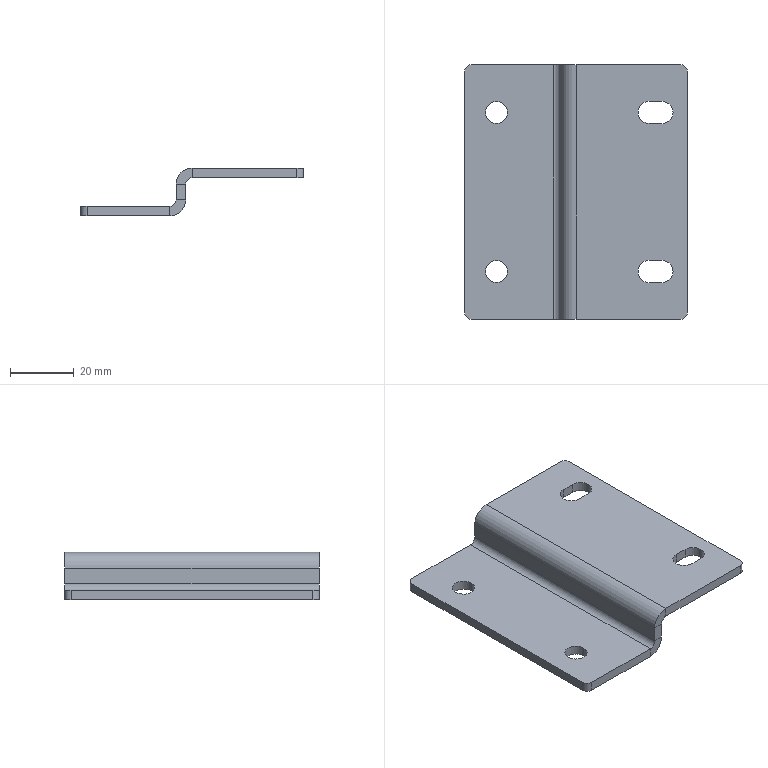Part | NX | features BREP 1 | 1 solid | 40 faces | box 70 x 80 x 15 mm | volume 18319 mm3 | plane 22 | cylinder 18 | commonest cylinder face diameters 7 x10 4 x6 10 x2
STEP:
#1=CARTESIAN_POINT('',(0.,-38.,-3.));
#2=VERTEX_POINT('',#1);
#3=CARTESIAN_POINT('',(-2.,-40.,-3.));
#4=VERTEX_POINT('',#3);
#5=CARTESIAN_POINT('',(-2.,-38.,-3.));
#6=DIRECTION('',(0.,0.,-1.));
#7=DIRECTION('',(1.,0.,0.));
#8=AXIS2_PLACEMENT_3D('',#5,#6,#7);
#9=CIRCLE('',#8,2.);
#10=EDGE_CURVE('',#2,#4,#9,.T.);
#11=ORIENTED_EDGE('',*,*,#10,.F.);
#12=CARTESIAN_POINT('',(0.,-38.,0.));
#13=VERTEX_POINT('',#12);
#14=CARTESIAN_POINT('',(0.,-38.,-3.));
#15=DIRECTION('',(0.,0.,-1.));
#16=VECTOR('',#15,1000.);
#17=LINE('',#14,#16);
#18=EDGE_CURVE('',#13,#2,#17,.T.);
#19=ORIENTED_EDGE('',*,*,#18,.F.);
#20=CARTESIAN_POINT('',(-2.,-40.,0.));
#21=VERTEX_POINT('',#20);
#22=CARTESIAN_POINT('',(-2.,-38.,0.));
#23=DIRECTION('',(0.,0.,1.));
#24=DIRECTION('',(1.,0.,0.));
#25=AXIS2_PLACEMENT_3D('',#22,#23,#24);
#26=CIRCLE('',#25,2.);
#27=EDGE_CURVE('',#21,#13,#26,.T.);
#28=ORIENTED_EDGE('',*,*,#27,.F.);
#29=CARTESIAN_POINT('',(-2.,-40.,-5.));
#30=DIRECTION('',(0.,0.,1.));
#31=VECTOR('',#30,1000.);
#32=LINE('',#29,#31);
#33=EDGE_CURVE('',#4,#21,#32,.T.);
#34=ORIENTED_EDGE('',*,*,#33,.F.);
#35=EDGE_LOOP('',(#11,#19,#28,#34));
#36=FACE_BOUND('',#35,.T.);
#37=CARTESIAN_POINT('',(-2.,-38.,-5.));
#38=DIRECTION('',(0.,0.,1.));
#39=DIRECTION('',(1.,0.,0.));
#40=AXIS2_PLACEMENT_3D('',#37,#38,#39);
#41=CYLINDRICAL_SURFACE('',#40,2.);
#42=ADVANCED_FACE('',(#36),#41,.T.);
#43=CARTESIAN_POINT('',(-70.,-38.,-12.));
#44=VERTEX_POINT('',#43);
#45=CARTESIAN_POINT('',(-68.,-40.,-12.));
#46=VERTEX_POINT('',#45);
#47=CARTESIAN_POINT('',(-68.,-38.,-12.));
#48=DIRECTION('',(0.,0.,1.));
#49=DIRECTION('',(1.,0.,0.));
#50=AXIS2_PLACEMENT_3D('',#47,#48,#49);
#51=CIRCLE('',#50,2.);
#52=EDGE_CURVE('',#44,#46,#51,.T.);
#53=ORIENTED_EDGE('',*,*,#52,.F.);
#54=CARTESIAN_POINT('',(-70.,-38.,-15.));
#55=VERTEX_POINT('',#54);
#56=CARTESIAN_POINT('',(-70.,-38.,-12.));
#57=DIRECTION('',(0.,0.,1.));
#58=VECTOR('',#57,1000.);
#59=LINE('',#56,#58);
#60=EDGE_CURVE('',#55,#44,#59,.T.);
#61=ORIENTED_EDGE('',*,*,#60,.F.);
#62=CARTESIAN_POINT('',(-68.,-40.,-15.));
#63=VERTEX_POINT('',#62);
#64=CARTESIAN_POINT('',(-68.,-38.,-15.));
#65=DIRECTION('',(0.,0.,-1.));
#66=DIRECTION('',(1.,0.,0.));
#67=AXIS2_PLACEMENT_3D('',#64,#65,#66);
#68=CIRCLE('',#67,2.);
#69=EDGE_CURVE('',#63,#55,#68,.T.);
#70=ORIENTED_EDGE('',*,*,#69,.F.);
#71=CARTESIAN_POINT('',(-68.,-40.,-10.));
#72=DIRECTION('',(0.,0.,-1.));
#73=VECTOR('',#72,1000.);
#74=LINE('',#71,#73);
#75=EDGE_CURVE('',#46,#63,#74,.T.);
#76=ORIENTED_EDGE('',*,*,#75,.F.);
#77=EDGE_LOOP('',(#53,#61,#70,#76));
#78=FACE_BOUND('',#77,.T.);
#79=CARTESIAN_POINT('',(-68.,-38.,-10.));
#80=DIRECTION('',(0.,0.,-1.));
#81=DIRECTION('',(-1.,0.,0.));
#82=AXIS2_PLACEMENT_3D('',#79,#80,#81);
#83=CYLINDRICAL_SURFACE('',#82,2.);
#84=ADVANCED_FACE('',(#78),#83,.T.);
#85=CARTESIAN_POINT('',(-68.,40.,-12.));
#86=VERTEX_POINT('',#85);
#87=CARTESIAN_POINT('',(-70.,38.,-12.));
#88=VERTEX_POINT('',#87);
#89=CARTESIAN_POINT('',(-68.,38.,-12.));
#90=DIRECTION('',(0.,0.,1.));
#91=DIRECTION('',(1.,0.,0.));
#92=AXIS2_PLACEMENT_3D('',#89,#90,#91);
#93=CIRCLE('',#92,2.);
#94=EDGE_CURVE('',#86,#88,#93,.T.);
#95=ORIENTED_EDGE('',*,*,#94,.F.);
#96=CARTESIAN_POINT('',(-68.,40.,-15.));
#97=VERTEX_POINT('',#96);
#98=CARTESIAN_POINT('',(-68.,40.,-10.));
#99=DIRECTION('',(0.,0.,1.));
#100=VECTOR('',#99,1000.);
#101=LINE('',#98,#100);
#102=EDGE_CURVE('',#97,#86,#101,.T.);
#103=ORIENTED_EDGE('',*,*,#102,.F.);
#104=CARTESIAN_POINT('',(-70.,38.,-15.));
#105=VERTEX_POINT('',#104);
#106=CARTESIAN_POINT('',(-68.,38.,-15.));
#107=DIRECTION('',(0.,0.,-1.));
#108=DIRECTION('',(1.,0.,0.));
#109=AXIS2_PLACEMENT_3D('',#106,#107,#108);
#110=CIRCLE('',#109,2.);
#111=EDGE_CURVE('',#105,#97,#110,.T.);
#112=ORIENTED_EDGE('',*,*,#111,.F.);
#113=CARTESIAN_POINT('',(-70.,38.,-12.));
#114=DIRECTION('',(0.,0.,-1.));
#115=VECTOR('',#114,1000.);
#116=LINE('',#113,#115);
#117=EDGE_CURVE('',#88,#105,#116,.T.);
#118=ORIENTED_EDGE('',*,*,#117,.F.);
#119=EDGE_LOOP('',(#95,#103,#112,#118));
#120=FACE_BOUND('',#119,.T.);
#121=CARTESIAN_POINT('',(-68.,38.,-12.));
#122=DIRECTION('',(0.,0.,-1.));
#123=DIRECTION('',(-1.,0.,0.));
#124=AXIS2_PLACEMENT_3D('',#121,#122,#123);
#125=CYLINDRICAL_SURFACE('',#124,2.);
#126=ADVANCED_FACE('',(#120),#125,.T.);
#127=CARTESIAN_POINT('',(-2.,40.,-3.));
#128=VERTEX_POINT('',#127);
#129=CARTESIAN_POINT('',(0.,38.,-3.));
#130=VERTEX_POINT('',#129);
#131=CARTESIAN_POINT('',(-2.,38.,-3.));
#132=DIRECTION('',(0.,0.,-1.));
#133=DIRECTION('',(1.,0.,0.));
#134=AXIS2_PLACEMENT_3D('',#131,#132,#133);
#135=CIRCLE('',#134,2.);
#136=EDGE_CURVE('',#128,#130,#135,.T.);
#137=ORIENTED_EDGE('',*,*,#136,.F.);
#138=CARTESIAN_POINT('',(-2.,40.,0.));
#139=VERTEX_POINT('',#138);
#140=CARTESIAN_POINT('',(-2.,40.,-3.));
#141=DIRECTION('',(0.,0.,-1.));
#142=VECTOR('',#141,1000.);
#143=LINE('',#140,#142);
#144=EDGE_CURVE('',#139,#128,#143,.T.);
#145=ORIENTED_EDGE('',*,*,#144,.F.);
#146=CARTESIAN_POINT('',(0.,38.,0.));
#147=VERTEX_POINT('',#146);
#148=CARTESIAN_POINT('',(-2.,38.,0.));
#149=DIRECTION('',(0.,0.,1.));
#150=DIRECTION('',(1.,0.,0.));
#151=AXIS2_PLACEMENT_3D('',#148,#149,#150);
#152=CIRCLE('',#151,2.);
#153=EDGE_CURVE('',#147,#139,#152,.T.);
#154=ORIENTED_EDGE('',*,*,#153,.F.);
#155=CARTESIAN_POINT('',(0.,38.,0.));
#156=DIRECTION('',(0.,0.,1.));
#157=VECTOR('',#156,1000.);
#158=LINE('',#155,#157);
#159=EDGE_CURVE('',#130,#147,#158,.T.);
#160=ORIENTED_EDGE('',*,*,#159,.F.);
#161=EDGE_LOOP('',(#137,#145,#154,#160));
#162=FACE_BOUND('',#161,.T.);
#163=CARTESIAN_POINT('',(-2.,38.,-3.));
#164=DIRECTION('',(0.,0.,-1.));
#165=DIRECTION('',(-1.,0.,0.));
#166=AXIS2_PLACEMENT_3D('',#163,#164,#165);
#167=CYLINDRICAL_SURFACE('',#166,2.);
#168=ADVANCED_FACE('',(#162),#167,.T.);
#169=CARTESIAN_POINT('',(-56.5,25.,-12.));
#170=VERTEX_POINT('',#169);
#171=CARTESIAN_POINT('',(-56.5,25.,-15.));
#172=VERTEX_POINT('',#171);
#173=CARTESIAN_POINT('',(-56.5,25.,-15.));
#174=DIRECTION('',(0.,0.,-1.));
#175=VECTOR('',#174,1000.);
#176=LINE('',#173,#175);
#177=EDGE_CURVE('',#170,#172,#176,.T.);
#178=ORIENTED_EDGE('',*,*,#177,.F.);
#179=CARTESIAN_POINT('',(-63.5,25.,-12.));
#180=VERTEX_POINT('',#179);
#181=CARTESIAN_POINT('',(-60.,25.,-12.));
#182=DIRECTION('',(0.,0.,1.));
#183=DIRECTION('',(1.,0.,0.));
#184=AXIS2_PLACEMENT_3D('',#181,#182,#183);
#185=CIRCLE('',#184,3.5);
#186=EDGE_CURVE('',#170,#180,#185,.T.);
#187=ORIENTED_EDGE('',*,*,#186,.T.);
#188=CARTESIAN_POINT('',(-63.5,25.,-15.));
#189=VERTEX_POINT('',#188);
#190=CARTESIAN_POINT('',(-63.5,25.,-15.));
#191=DIRECTION('',(0.,0.,-1.));
#192=VECTOR('',#191,1000.);
#193=LINE('',#190,#192);
#194=EDGE_CURVE('',#180,#189,#193,.T.);
#195=ORIENTED_EDGE('',*,*,#194,.T.);
#196=CARTESIAN_POINT('',(-60.,25.,-15.));
#197=DIRECTION('',(0.,0.,-1.));
#198=DIRECTION('',(-1.,0.,0.));
#199=AXIS2_PLACEMENT_3D('',#196,#197,#198);
#200=CIRCLE('',#199,3.5);
#201=EDGE_CURVE('',#189,#172,#200,.T.);
#202=ORIENTED_EDGE('',*,*,#201,.T.);
#203=EDGE_LOOP('',(#178,#187,#195,#202));
#204=FACE_BOUND('',#203,.T.);
#205=CARTESIAN_POINT('',(-60.,25.,-15.));
#206=DIRECTION('',(0.,0.,-1.));
#207=DIRECTION('',(-1.,0.,0.));
#208=AXIS2_PLACEMENT_3D('',#205,#206,#207);
#209=CYLINDRICAL_SURFACE('',#208,3.5);
#210=ADVANCED_FACE('',(#204),#209,.F.);
#211=CARTESIAN_POINT('',(-56.5,-25.,-12.));
#212=VERTEX_POINT('',#211);
#213=CARTESIAN_POINT('',(-56.5,-25.,-15.));
#214=VERTEX_POINT('',#213);
#215=CARTESIAN_POINT('',(-56.5,-25.,-15.));
#216=DIRECTION('',(0.,0.,-1.));
#217=VECTOR('',#216,1000.);
#218=LINE('',#215,#217);
#219=EDGE_CURVE('',#212,#214,#218,.T.);
#220=ORIENTED_EDGE('',*,*,#219,.F.);
#221=CARTESIAN_POINT('',(-63.5,-25.,-12.));
#222=VERTEX_POINT('',#221);
#223=CARTESIAN_POINT('',(-60.,-25.,-12.));
#224=DIRECTION('',(0.,0.,1.));
#225=DIRECTION('',(1.,0.,0.));
#226=AXIS2_PLACEMENT_3D('',#223,#224,#225);
#227=CIRCLE('',#226,3.5);
#228=EDGE_CURVE('',#212,#222,#227,.T.);
#229=ORIENTED_EDGE('',*,*,#228,.T.);
#230=CARTESIAN_POINT('',(-63.5,-25.,-15.));
#231=VERTEX_POINT('',#230);
#232=CARTESIAN_POINT('',(-63.5,-25.,-15.));
#233=DIRECTION('',(0.,0.,-1.));
#234=VECTOR('',#233,1000.);
#235=LINE('',#232,#234);
#236=EDGE_CURVE('',#222,#231,#235,.T.);
#237=ORIENTED_EDGE('',*,*,#236,.T.);
#238=CARTESIAN_POINT('',(-60.,-25.,-15.));
#239=DIRECTION('',(0.,0.,-1.));
#240=DIRECTION('',(-1.,0.,0.));
#241=AXIS2_PLACEMENT_3D('',#238,#239,#240);
#242=CIRCLE('',#241,3.5);
#243=EDGE_CURVE('',#231,#214,#242,.T.);
#244=ORIENTED_EDGE('',*,*,#243,.T.);
#245=EDGE_LOOP('',(#220,#229,#237,#244));
#246=FACE_BOUND('',#245,.T.);
#247=CARTESIAN_POINT('',(-60.,-25.,-15.));
#248=DIRECTION('',(0.,0.,-1.));
#249=DIRECTION('',(-1.,0.,0.));
#250=AXIS2_PLACEMENT_3D('',#247,#248,#249);
#251=CYLINDRICAL_SURFACE('',#250,3.5);
#252=ADVANCED_FACE('',(#246),#251,.F.);
#253=CARTESIAN_POINT('',(-12.,21.5,-3.));
#254=VERTEX_POINT('',#253);
#255=CARTESIAN_POINT('',(-12.,21.5,0.));
#256=VERTEX_POINT('',#255);
#257=CARTESIAN_POINT('',(-12.,21.5,-15.));
#258=DIRECTION('',(0.,0.,1.));
#259=VECTOR('',#258,1000.);
#260=LINE('',#257,#259);
#261=EDGE_CURVE('',#254,#256,#260,.T.);
#262=ORIENTED_EDGE('',*,*,#261,.T.);
#263=CARTESIAN_POINT('',(-8.,21.5,0.));
#264=VERTEX_POINT('',#263);
#265=CARTESIAN_POINT('',(-12.,21.5,0.));
#266=DIRECTION('',(1.,0.,0.));
#267=VECTOR('',#266,1000.);
#268=LINE('',#265,#267);
#269=EDGE_CURVE('',#256,#264,#268,.T.);
#270=ORIENTED_EDGE('',*,*,#269,.T.);
#271=CARTESIAN_POINT('',(-8.,21.5,-3.));
#272=VERTEX_POINT('',#271);
#273=CARTESIAN_POINT('',(-8.,21.5,-15.));
#274=DIRECTION('',(0.,0.,1.));
#275=VECTOR('',#274,1000.);
#276=LINE('',#273,#275);
#277=EDGE_CURVE('',#272,#264,#276,.T.);
#278=ORIENTED_EDGE('',*,*,#277,.F.);
#279=CARTESIAN_POINT('',(0.,21.5,-3.));
#280=DIRECTION('',(1.,0.,0.));
#281=VECTOR('',#280,1000.);
#282=LINE('',#279,#281);
#283=EDGE_CURVE('',#254,#272,#282,.T.);
#284=ORIENTED_EDGE('',*,*,#283,.F.);
#285=EDGE_LOOP('',(#262,#270,#278,#284));
#286=FACE_BOUND('',#285,.T.);
#287=CARTESIAN_POINT('',(-12.,21.5,-15.));
#288=DIRECTION('',(0.,-1.,0.));
#289=DIRECTION('',(0.,0.,-1.));
#290=AXIS2_PLACEMENT_3D('',#287,#288,#289);
#291=PLANE('',#290);
#292=ADVANCED_FACE('',(#286),#291,.F.);
#293=CARTESIAN_POINT('',(-4.5,25.,-3.));
#294=VERTEX_POINT('',#293);
#295=CARTESIAN_POINT('',(-4.5,25.,0.));
#296=VERTEX_POINT('',#295);
#297=CARTESIAN_POINT('',(-4.5,25.,-15.));
#298=DIRECTION('',(0.,0.,1.));
#299=VECTOR('',#298,1000.);
#300=LINE('',#297,#299);
#301=EDGE_CURVE('',#294,#296,#300,.T.);
#302=ORIENTED_EDGE('',*,*,#301,.F.);
#303=CARTESIAN_POINT('',(-8.,25.,-3.));
#304=DIRECTION('',(0.,0.,1.));
#305=DIRECTION('',(1.,0.,0.));
#306=AXIS2_PLACEMENT_3D('',#303,#304,#305);
#307=CIRCLE('',#306,3.5);
#308=EDGE_CURVE('',#272,#294,#307,.T.);
#309=ORIENTED_EDGE('',*,*,#308,.F.);
#310=ORIENTED_EDGE('',*,*,#277,.T.);
#311=CARTESIAN_POINT('',(-8.,25.,0.));
#312=DIRECTION('',(0.,0.,1.));
#313=DIRECTION('',(1.,0.,0.));
#314=AXIS2_PLACEMENT_3D('',#311,#312,#313);
#315=CIRCLE('',#314,3.5);
#316=EDGE_CURVE('',#264,#296,#315,.T.);
#317=ORIENTED_EDGE('',*,*,#316,.T.);
#318=EDGE_LOOP('',(#302,#309,#310,#317));
#319=FACE_BOUND('',#318,.T.);
#320=CARTESIAN_POINT('',(-8.,25.,-15.));
#321=DIRECTION('',(0.,0.,1.));
#322=DIRECTION('',(1.,0.,0.));
#323=AXIS2_PLACEMENT_3D('',#320,#321,#322);
#324=CYLINDRICAL_SURFACE('',#323,3.5);
#325=ADVANCED_FACE('',(#319),#324,.F.);
#326=CARTESIAN_POINT('',(-8.,28.5,-3.));
#327=VERTEX_POINT('',#326);
#328=CARTESIAN_POINT('',(-8.,28.5,0.));
#329=VERTEX_POINT('',#328);
#330=CARTESIAN_POINT('',(-8.,28.5,-15.));
#331=DIRECTION('',(0.,0.,1.));
#332=VECTOR('',#331,1000.);
#333=LINE('',#330,#332);
#334=EDGE_CURVE('',#327,#329,#333,.T.);
#335=ORIENTED_EDGE('',*,*,#334,.T.);
#336=CARTESIAN_POINT('',(-12.,28.5,0.));
#337=VERTEX_POINT('',#336);
#338=CARTESIAN_POINT('',(-12.,28.5,0.));
#339=DIRECTION('',(-1.,0.,0.));
#340=VECTOR('',#339,1000.);
#341=LINE('',#338,#340);
#342=EDGE_CURVE('',#329,#337,#341,.T.);
#343=ORIENTED_EDGE('',*,*,#342,.T.);
#344=CARTESIAN_POINT('',(-12.,28.5,-3.));
#345=VERTEX_POINT('',#344);
#346=CARTESIAN_POINT('',(-12.,28.5,-15.));
#347=DIRECTION('',(0.,0.,1.));
#348=VECTOR('',#347,1000.);
#349=LINE('',#346,#348);
#350=EDGE_CURVE('',#345,#337,#349,.T.);
#351=ORIENTED_EDGE('',*,*,#350,.F.);
#352=CARTESIAN_POINT('',(0.,28.5,-3.));
#353=DIRECTION('',(-1.,0.,0.));
#354=VECTOR('',#353,1000.);
#355=LINE('',#352,#354);
#356=EDGE_CURVE('',#327,#345,#355,.T.);
#357=ORIENTED_EDGE('',*,*,#356,.F.);
#358=EDGE_LOOP('',(#335,#343,#351,#357));
#359=FACE_BOUND('',#358,.T.);
#360=CARTESIAN_POINT('',(-12.,28.5,-15.));
#361=DIRECTION('',(0.,1.,0.));
#362=DIRECTION('',(-1.,0.,0.));
#363=AXIS2_PLACEMENT_3D('',#360,#361,#362);
#364=PLANE('',#363);
#365=ADVANCED_FACE('',(#359),#364,.F.);
#366=ORIENTED_EDGE('',*,*,#350,.T.);
#367=CARTESIAN_POINT('',(-12.,25.,0.));
#368=DIRECTION('',(0.,0.,1.));
#369=DIRECTION('',(1.,0.,0.));
#370=AXIS2_PLACEMENT_3D('',#367,#368,#369);
#371=CIRCLE('',#370,3.5);
#372=EDGE_CURVE('',#337,#256,#371,.T.);
#373=ORIENTED_EDGE('',*,*,#372,.T.);
#374=ORIENTED_EDGE('',*,*,#261,.F.);
#375=CARTESIAN_POINT('',(-12.,25.,-3.));
#376=DIRECTION('',(0.,0.,1.));
#377=DIRECTION('',(1.,0.,0.));
#378=AXIS2_PLACEMENT_3D('',#375,#376,#377);
#379=CIRCLE('',#378,3.5);
#380=EDGE_CURVE('',#345,#254,#379,.T.);
#381=ORIENTED_EDGE('',*,*,#380,.F.);
#382=EDGE_LOOP('',(#366,#373,#374,#381));
#383=FACE_BOUND('',#382,.T.);
#384=CARTESIAN_POINT('',(-12.,25.,-15.));
#385=DIRECTION('',(0.,0.,1.));
#386=DIRECTION('',(1.,0.,0.));
#387=AXIS2_PLACEMENT_3D('',#384,#385,#386);
#388=CYLINDRICAL_SURFACE('',#387,3.5);
#389=ADVANCED_FACE('',(#383),#388,.F.);
#390=CARTESIAN_POINT('',(-8.,-21.5,-3.));
#391=VERTEX_POINT('',#390);
#392=CARTESIAN_POINT('',(-8.,-21.5,0.));
#393=VERTEX_POINT('',#392);
#394=CARTESIAN_POINT('',(-8.,-21.5,-15.));
#395=DIRECTION('',(0.,0.,1.));
#396=VECTOR('',#395,1000.);
#397=LINE('',#394,#396);
#398=EDGE_CURVE('',#391,#393,#397,.T.);
#399=ORIENTED_EDGE('',*,*,#398,.T.);
#400=CARTESIAN_POINT('',(-12.,-21.5,0.));
#401=VERTEX_POINT('',#400);
#402=CARTESIAN_POINT('',(-8.,-21.5,0.));
#403=DIRECTION('',(-1.,0.,0.));
#404=VECTOR('',#403,1000.);
#405=LINE('',#402,#404);
#406=EDGE_CURVE('',#393,#401,#405,.T.);
#407=ORIENTED_EDGE('',*,*,#406,.T.);
#408=CARTESIAN_POINT('',(-12.,-21.5,-3.));
#409=VERTEX_POINT('',#408);
#410=CARTESIAN_POINT('',(-12.,-21.5,-15.));
#411=DIRECTION('',(0.,0.,1.));
#412=VECTOR('',#411,1000.);
#413=LINE('',#410,#412);
#414=EDGE_CURVE('',#409,#401,#413,.T.);
#415=ORIENTED_EDGE('',*,*,#414,.F.);
#416=CARTESIAN_POINT('',(0.,-21.5,-3.));
#417=DIRECTION('',(-1.,0.,0.));
#418=VECTOR('',#417,1000.);
#419=LINE('',#416,#418);
#420=EDGE_CURVE('',#391,#409,#419,.T.);
#421=ORIENTED_EDGE('',*,*,#420,.F.);
#422=EDGE_LOOP('',(#399,#407,#415,#421));
#423=FACE_BOUND('',#422,.T.);
#424=CARTESIAN_POINT('',(-8.,-21.5,-15.));
#425=DIRECTION('',(0.,1.,0.));
#426=DIRECTION('',(0.,0.,1.));
#427=AXIS2_PLACEMENT_3D('',#424,#425,#426);
#428=PLANE('',#427);
#429=ADVANCED_FACE('',(#423),#428,.F.);
#430=ORIENTED_EDGE('',*,*,#414,.T.);
#431=CARTESIAN_POINT('',(-12.,-28.5,0.));
#432=VERTEX_POINT('',#431);
#433=CARTESIAN_POINT('',(-12.,-25.,0.));
#434=DIRECTION('',(0.,0.,1.));
#435=DIRECTION('',(1.,0.,0.));
#436=AXIS2_PLACEMENT_3D('',#433,#434,#435);
#437=CIRCLE('',#436,3.5);
#438=EDGE_CURVE('',#401,#432,#437,.T.);
#439=ORIENTED_EDGE('',*,*,#438,.T.);
#440=CARTESIAN_POINT('',(-12.,-28.5,-3.));
#441=VERTEX_POINT('',#440);
#442=CARTESIAN_POINT('',(-12.,-28.5,-15.));
#443=DIRECTION('',(0.,0.,1.));
#444=VECTOR('',#443,1000.);
#445=LINE('',#442,#444);
#446=EDGE_CURVE('',#441,#432,#445,.T.);
#447=ORIENTED_EDGE('',*,*,#446,.F.);
#448=CARTESIAN_POINT('',(-12.,-25.,-3.));
#449=DIRECTION('',(0.,0.,1.));
#450=DIRECTION('',(1.,0.,0.));
#451=AXIS2_PLACEMENT_3D('',#448,#449,#450);
#452=CIRCLE('',#451,3.5);
#453=EDGE_CURVE('',#409,#441,#452,.T.);
#454=ORIENTED_EDGE('',*,*,#453,.F.);
#455=EDGE_LOOP('',(#430,#439,#447,#454));
#456=FACE_BOUND('',#455,.T.);
#457=CARTESIAN_POINT('',(-12.,-25.,-15.));
#458=DIRECTION('',(0.,0.,1.));
#459=DIRECTION('',(1.,0.,0.));
#460=AXIS2_PLACEMENT_3D('',#457,#458,#459);
#461=CYLINDRICAL_SURFACE('',#460,3.5);
#462=ADVANCED_FACE('',(#456),#461,.F.);
#463=ORIENTED_EDGE('',*,*,#446,.T.);
#464=CARTESIAN_POINT('',(-8.,-28.5,0.));
#465=VERTEX_POINT('',#464);
#466=CARTESIAN_POINT('',(-8.,-28.5,0.));
#467=DIRECTION('',(1.,0.,0.));
#468=VECTOR('',#467,1000.);
#469=LINE('',#466,#468);
#470=EDGE_CURVE('',#432,#465,#469,.T.);
#471=ORIENTED_EDGE('',*,*,#470,.T.);
#472=CARTESIAN_POINT('',(-8.,-28.5,-3.));
#473=VERTEX_POINT('',#472);
#474=CARTESIAN_POINT('',(-8.,-28.5,-15.));
#475=DIRECTION('',(0.,0.,1.));
#476=VECTOR('',#475,1000.);
#477=LINE('',#474,#476);
#478=EDGE_CURVE('',#473,#465,#477,.T.);
#479=ORIENTED_EDGE('',*,*,#478,.F.);
#480=CARTESIAN_POINT('',(0.,-28.5,-3.));
#481=DIRECTION('',(1.,0.,0.));
#482=VECTOR('',#481,1000.);
#483=LINE('',#480,#482);
#484=EDGE_CURVE('',#441,#473,#483,.T.);
#485=ORIENTED_EDGE('',*,*,#484,.F.);
#486=EDGE_LOOP('',(#463,#471,#479,#485));
#487=FACE_BOUND('',#486,.T.);
#488=CARTESIAN_POINT('',(-8.,-28.5,-15.));
#489=DIRECTION('',(0.,-1.,0.));
#490=DIRECTION('',(0.,0.,-1.));
#491=AXIS2_PLACEMENT_3D('',#488,#489,#490);
#492=PLANE('',#491);
#493=ADVANCED_FACE('',(#487),#492,.F.);
#494=CARTESIAN_POINT('',(-4.5,-25.,-3.));
#495=VERTEX_POINT('',#494);
#496=CARTESIAN_POINT('',(-4.5,-25.,0.));
#497=VERTEX_POINT('',#496);
#498=CARTESIAN_POINT('',(-4.5,-25.,-15.));
#499=DIRECTION('',(0.,0.,1.));
#500=VECTOR('',#499,1000.);
#501=LINE('',#498,#500);
#502=EDGE_CURVE('',#495,#497,#501,.T.);
#503=ORIENTED_EDGE('',*,*,#502,.F.);
#504=CARTESIAN_POINT('',(-8.,-25.,-3.));
#505=DIRECTION('',(0.,0.,1.));
#506=DIRECTION('',(1.,0.,0.));
#507=AXIS2_PLACEMENT_3D('',#504,#505,#506);
#508=CIRCLE('',#507,3.5);
#509=EDGE_CURVE('',#473,#495,#508,.T.);
#510=ORIENTED_EDGE('',*,*,#509,.F.);
#511=ORIENTED_EDGE('',*,*,#478,.T.);
#512=CARTESIAN_POINT('',(-8.,-25.,0.));
#513=DIRECTION('',(0.,0.,1.));
#514=DIRECTION('',(1.,0.,0.));
#515=AXIS2_PLACEMENT_3D('',#512,#513,#514);
#516=CIRCLE('',#515,3.5);
#517=EDGE_CURVE('',#465,#497,#516,.T.);
#518=ORIENTED_EDGE('',*,*,#517,.T.);
#519=EDGE_LOOP('',(#503,#510,#511,#518));
#520=FACE_BOUND('',#519,.T.);
#521=CARTESIAN_POINT('',(-8.,-25.,-15.));
#522=DIRECTION('',(0.,0.,1.));
#523=DIRECTION('',(1.,0.,0.));
#524=AXIS2_PLACEMENT_3D('',#521,#522,#523);
#525=CYLINDRICAL_SURFACE('',#524,3.5);
#526=ADVANCED_FACE('',(#520),#525,.F.);
#527=CARTESIAN_POINT('',(-42.,-40.,-12.));
#528=VERTEX_POINT('',#527);
#529=CARTESIAN_POINT('',(-40.,-40.,-12.));
#530=DIRECTION('',(-1.,0.,0.));
#531=VECTOR('',#530,1000.);
#532=LINE('',#529,#531);
#533=EDGE_CURVE('',#528,#46,#532,.T.);
#534=ORIENTED_EDGE('',*,*,#533,.T.);
#535=ORIENTED_EDGE('',*,*,#75,.T.);
#536=CARTESIAN_POINT('',(-42.,-40.,-15.));
#537=VERTEX_POINT('',#536);
#538=CARTESIAN_POINT('',(-40.,-40.,-15.));
#539=DIRECTION('',(-1.,0.,0.));
#540=VECTOR('',#539,1000.);
#541=LINE('',#538,#540);
#542=EDGE_CURVE('',#537,#63,#541,.T.);
#543=ORIENTED_EDGE('',*,*,#542,.F.);
#544=CARTESIAN_POINT('',(-42.,-40.,-15.));
#545=DIRECTION('',(0.,0.,1.));
#546=VECTOR('',#545,1000.);
#547=LINE('',#544,#546);
#548=EDGE_CURVE('',#537,#528,#547,.T.);
#549=ORIENTED_EDGE('',*,*,#548,.T.);
#550=EDGE_LOOP('',(#534,#535,#543,#549));
#551=FACE_BOUND('',#550,.T.);
#552=CARTESIAN_POINT('',(-42.,-40.,-10.));
#553=DIRECTION('',(0.,-1.,0.));
#554=DIRECTION('',(-1.,0.,0.));
#555=AXIS2_PLACEMENT_3D('',#552,#553,#554);
#556=PLANE('',#555);
#557=ADVANCED_FACE('',(#551),#556,.T.);
#558=CARTESIAN_POINT('',(-35.,40.,0.));
#559=VERTEX_POINT('',#558);
#560=CARTESIAN_POINT('',(0.,40.,0.));
#561=DIRECTION('',(-1.,0.,0.));
#562=VECTOR('',#561,1000.);
#563=LINE('',#560,#562);
#564=EDGE_CURVE('',#139,#559,#563,.T.);
#565=ORIENTED_EDGE('',*,*,#564,.F.);
#566=ORIENTED_EDGE('',*,*,#144,.T.);
#567=CARTESIAN_POINT('',(-35.,40.,-3.));
#568=VERTEX_POINT('',#567);
#569=CARTESIAN_POINT('',(0.,40.,-3.));
#570=DIRECTION('',(-1.,0.,0.));
#571=VECTOR('',#570,1000.);
#572=LINE('',#569,#571);
#573=EDGE_CURVE('',#128,#568,#572,.T.);
#574=ORIENTED_EDGE('',*,*,#573,.T.);
#575=CARTESIAN_POINT('',(-35.,40.,-3.));
#576=DIRECTION('',(0.,0.,1.));
#577=VECTOR('',#576,1000.);
#578=LINE('',#575,#577);
#579=EDGE_CURVE('',#568,#559,#578,.T.);
#580=ORIENTED_EDGE('',*,*,#579,.T.);
#581=EDGE_LOOP('',(#565,#566,#574,#580));
#582=FACE_BOUND('',#581,.T.);
#583=CARTESIAN_POINT('',(-42.,40.,-10.));
#584=DIRECTION('',(0.,-1.,0.));
#585=DIRECTION('',(-1.,0.,0.));
#586=AXIS2_PLACEMENT_3D('',#583,#584,#585);
#587=PLANE('',#586);
#588=ADVANCED_FACE('',(#582),#587,.F.);
#589=CARTESIAN_POINT('',(-37.,-40.,-10.));
#590=VERTEX_POINT('',#589);
#591=CARTESIAN_POINT('',(-42.,-40.,-10.));
#592=DIRECTION('',(0.,1.,0.));
#593=DIRECTION('',(1.,0.,0.));
#594=AXIS2_PLACEMENT_3D('',#591,#592,#593);
#595=CIRCLE('',#594,5.);
#596=EDGE_CURVE('',#590,#537,#595,.T.);
#597=ORIENTED_EDGE('',*,*,#596,.T.);
#598=CARTESIAN_POINT('',(-42.,40.,-15.));
#599=VERTEX_POINT('',#598);
#600=CARTESIAN_POINT('',(-42.,40.,-15.));
#601=DIRECTION('',(0.,-1.,0.));
#602=VECTOR('',#601,1000.);
#603=LINE('',#600,#602);
#604=EDGE_CURVE('',#599,#537,#603,.T.);
#605=ORIENTED_EDGE('',*,*,#604,.F.);
#606=CARTESIAN_POINT('',(-37.,40.,-10.));
#607=VERTEX_POINT('',#606);
#608=CARTESIAN_POINT('',(-42.,40.,-10.));
#609=DIRECTION('',(0.,1.,0.));
#610=DIRECTION('',(1.,0.,0.));
#611=AXIS2_PLACEMENT_3D('',#608,#609,#610);
#612=CIRCLE('',#611,5.);
#613=EDGE_CURVE('',#607,#599,#612,.T.);
#614=ORIENTED_EDGE('',*,*,#613,.F.);
#615=CARTESIAN_POINT('',(-37.,40.,-10.));
#616=DIRECTION('',(0.,-1.,0.));
#617=VECTOR('',#616,1000.);
#618=LINE('',#615,#617);
#619=EDGE_CURVE('',#607,#590,#618,.T.);
#620=ORIENTED_EDGE('',*,*,#619,.T.);
#621=EDGE_LOOP('',(#597,#605,#614,#620));
#622=FACE_BOUND('',#621,.T.);
#623=CARTESIAN_POINT('',(-42.,40.,-10.));
#624=DIRECTION('',(0.,-1.,0.));
#625=DIRECTION('',(0.,0.,-1.));
#626=AXIS2_PLACEMENT_3D('',#623,#624,#625);
#627=CYLINDRICAL_SURFACE('',#626,5.);
#628=ADVANCED_FACE('',(#622),#627,.T.);
#629=CARTESIAN_POINT('',(-37.,-40.,-5.));
#630=VERTEX_POINT('',#629);
#631=CARTESIAN_POINT('',(-37.,-40.,0.));
#632=DIRECTION('',(0.,0.,-1.));
#633=VECTOR('',#632,1000.);
#634=LINE('',#631,#633);
#635=EDGE_CURVE('',#630,#590,#634,.T.);
#636=ORIENTED_EDGE('',*,*,#635,.T.);
#637=ORIENTED_EDGE('',*,*,#619,.F.);
#638=CARTESIAN_POINT('',(-37.,40.,-5.));
#639=VERTEX_POINT('',#638);
#640=CARTESIAN_POINT('',(-37.,40.,0.));
#641=DIRECTION('',(0.,0.,-1.));
#642=VECTOR('',#641,1000.);
#643=LINE('',#640,#642);
#644=EDGE_CURVE('',#639,#607,#643,.T.);
#645=ORIENTED_EDGE('',*,*,#644,.F.);
#646=CARTESIAN_POINT('',(-37.,40.,-5.));
#647=DIRECTION('',(0.,-1.,0.));
#648=VECTOR('',#647,1000.);
#649=LINE('',#646,#648);
#650=EDGE_CURVE('',#639,#630,#649,.T.);
#651=ORIENTED_EDGE('',*,*,#650,.T.);
#652=EDGE_LOOP('',(#636,#637,#645,#651));
#653=FACE_BOUND('',#652,.T.);
#654=CARTESIAN_POINT('',(-37.,40.,0.));
#655=DIRECTION('',(-1.,0.,0.));
#656=DIRECTION('',(0.,0.,1.));
#657=AXIS2_PLACEMENT_3D('',#654,#655,#656);
#658=PLANE('',#657);
#659=ADVANCED_FACE('',(#653),#658,.F.);
#660=CARTESIAN_POINT('',(-35.,-40.,-3.));
#661=VERTEX_POINT('',#660);
#662=CARTESIAN_POINT('',(-35.,-40.,-5.));
#663=DIRECTION('',(0.,-1.,0.));
#664=DIRECTION('',(1.,0.,0.));
#665=AXIS2_PLACEMENT_3D('',#662,#663,#664);
#666=CIRCLE('',#665,2.);
#667=EDGE_CURVE('',#661,#630,#666,.T.);
#668=ORIENTED_EDGE('',*,*,#667,.T.);
#669=ORIENTED_EDGE('',*,*,#650,.F.);
#670=CARTESIAN_POINT('',(-35.,40.,-5.));
#671=DIRECTION('',(0.,-1.,0.));
#672=DIRECTION('',(1.,0.,0.));
#673=AXIS2_PLACEMENT_3D('',#670,#671,#672);
#674=CIRCLE('',#673,2.);
#675=EDGE_CURVE('',#568,#639,#674,.T.);
#676=ORIENTED_EDGE('',*,*,#675,.F.);
#677=CARTESIAN_POINT('',(-35.,40.,-3.));
#678=DIRECTION('',(0.,-1.,0.));
#679=VECTOR('',#678,1000.);
#680=LINE('',#677,#679);
#681=EDGE_CURVE('',#568,#661,#680,.T.);
#682=ORIENTED_EDGE('',*,*,#681,.T.);
#683=EDGE_LOOP('',(#668,#669,#676,#682));
#684=FACE_BOUND('',#683,.T.);
#685=CARTESIAN_POINT('',(-35.,40.,-5.));
#686=DIRECTION('',(0.,-1.,0.));
#687=DIRECTION('',(0.,0.,-1.));
#688=AXIS2_PLACEMENT_3D('',#685,#686,#687);
#689=CYLINDRICAL_SURFACE('',#688,2.);
#690=ADVANCED_FACE('',(#684),#689,.F.);
#691=ORIENTED_EDGE('',*,*,#573,.F.);
#692=ORIENTED_EDGE('',*,*,#136,.T.);
#693=CARTESIAN_POINT('',(0.,40.,-3.));
#694=DIRECTION('',(0.,-1.,0.));
#695=VECTOR('',#694,1000.);
#696=LINE('',#693,#695);
#697=EDGE_CURVE('',#130,#2,#696,.T.);
#698=ORIENTED_EDGE('',*,*,#697,.T.);
#699=ORIENTED_EDGE('',*,*,#10,.T.);
#700=CARTESIAN_POINT('',(0.,-40.,-3.));
#701=DIRECTION('',(-1.,0.,0.));
#702=VECTOR('',#701,1000.);
#703=LINE('',#700,#702);
#704=EDGE_CURVE('',#4,#661,#703,.T.);
#705=ORIENTED_EDGE('',*,*,#704,.T.);
#706=ORIENTED_EDGE('',*,*,#681,.F.);
#707=EDGE_LOOP('',(#691,#692,#698,#699,#705,#706));
#708=FACE_BOUND('',#707,.T.);
#709=ORIENTED_EDGE('',*,*,#484,.T.);
#710=ORIENTED_EDGE('',*,*,#509,.T.);
#711=CARTESIAN_POINT('',(-8.,-25.,-3.));
#712=DIRECTION('',(0.,0.,1.));
#713=DIRECTION('',(1.,0.,0.));
#714=AXIS2_PLACEMENT_3D('',#711,#712,#713);
#715=CIRCLE('',#714,3.5);
#716=EDGE_CURVE('',#495,#391,#715,.T.);
#717=ORIENTED_EDGE('',*,*,#716,.T.);
#718=ORIENTED_EDGE('',*,*,#420,.T.);
#719=ORIENTED_EDGE('',*,*,#453,.T.);
#720=EDGE_LOOP('',(#709,#710,#717,#718,#719));
#721=FACE_BOUND('',#720,.T.);
#722=ORIENTED_EDGE('',*,*,#356,.T.);
#723=ORIENTED_EDGE('',*,*,#380,.T.);
#724=ORIENTED_EDGE('',*,*,#283,.T.);
#725=ORIENTED_EDGE('',*,*,#308,.T.);
#726=CARTESIAN_POINT('',(-8.,25.,-3.));
#727=DIRECTION('',(0.,0.,1.));
#728=DIRECTION('',(1.,0.,0.));
#729=AXIS2_PLACEMENT_3D('',#726,#727,#728);
#730=CIRCLE('',#729,3.5);
#731=EDGE_CURVE('',#294,#327,#730,.T.);
#732=ORIENTED_EDGE('',*,*,#731,.T.);
#733=EDGE_LOOP('',(#722,#723,#724,#725,#732));
#734=FACE_BOUND('',#733,.T.);
#735=CARTESIAN_POINT('',(0.,40.,-3.));
#736=DIRECTION('',(0.,0.,1.));
#737=DIRECTION('',(1.,0.,0.));
#738=AXIS2_PLACEMENT_3D('',#735,#736,#737);
#739=PLANE('',#738);
#740=ADVANCED_FACE('',(#708,#721,#734),#739,.F.);
#741=ORIENTED_EDGE('',*,*,#697,.F.);
#742=ORIENTED_EDGE('',*,*,#159,.T.);
#743=CARTESIAN_POINT('',(0.,40.,0.));
#744=DIRECTION('',(0.,-1.,0.));
#745=VECTOR('',#744,1000.);
#746=LINE('',#743,#745);
#747=EDGE_CURVE('',#147,#13,#746,.T.);
#748=ORIENTED_EDGE('',*,*,#747,.T.);
#749=ORIENTED_EDGE('',*,*,#18,.T.);
#750=EDGE_LOOP('',(#741,#742,#748,#749));
#751=FACE_BOUND('',#750,.T.);
#752=CARTESIAN_POINT('',(0.,40.,-3.));
#753=DIRECTION('',(1.,0.,0.));
#754=DIRECTION('',(0.,0.,-1.));
#755=AXIS2_PLACEMENT_3D('',#752,#753,#754);
#756=PLANE('',#755);
#757=ADVANCED_FACE('',(#751),#756,.T.);
#758=ORIENTED_EDGE('',*,*,#747,.F.);
#759=ORIENTED_EDGE('',*,*,#153,.T.);
#760=ORIENTED_EDGE('',*,*,#564,.T.);
#761=CARTESIAN_POINT('',(-35.,-40.,0.));
#762=VERTEX_POINT('',#761);
#763=CARTESIAN_POINT('',(-35.,40.,0.));
#764=DIRECTION('',(0.,-1.,0.));
#765=VECTOR('',#764,1000.);
#766=LINE('',#763,#765);
#767=EDGE_CURVE('',#559,#762,#766,.T.);
#768=ORIENTED_EDGE('',*,*,#767,.T.);
#769=CARTESIAN_POINT('',(0.,-40.,0.));
#770=DIRECTION('',(-1.,0.,0.));
#771=VECTOR('',#770,1000.);
#772=LINE('',#769,#771);
#773=EDGE_CURVE('',#21,#762,#772,.T.);
#774=ORIENTED_EDGE('',*,*,#773,.F.);
#775=ORIENTED_EDGE('',*,*,#27,.T.);
#776=EDGE_LOOP('',(#758,#759,#760,#768,#774,#775));
#777=FACE_BOUND('',#776,.T.);
#778=ORIENTED_EDGE('',*,*,#517,.F.);
#779=ORIENTED_EDGE('',*,*,#470,.F.);
#780=ORIENTED_EDGE('',*,*,#438,.F.);
#781=ORIENTED_EDGE('',*,*,#406,.F.);
#782=CARTESIAN_POINT('',(-8.,-25.,0.));
#783=DIRECTION('',(0.,0.,1.));
#784=DIRECTION('',(1.,0.,0.));
#785=AXIS2_PLACEMENT_3D('',#782,#783,#784);
#786=CIRCLE('',#785,3.5);
#787=EDGE_CURVE('',#497,#393,#786,.T.);
#788=ORIENTED_EDGE('',*,*,#787,.F.);
#789=EDGE_LOOP('',(#778,#779,#780,#781,#788));
#790=FACE_BOUND('',#789,.T.);
#791=ORIENTED_EDGE('',*,*,#372,.F.);
#792=ORIENTED_EDGE('',*,*,#342,.F.);
#793=CARTESIAN_POINT('',(-8.,25.,0.));
#794=DIRECTION('',(0.,0.,1.));
#795=DIRECTION('',(1.,0.,0.));
#796=AXIS2_PLACEMENT_3D('',#793,#794,#795);
#797=CIRCLE('',#796,3.5);
#798=EDGE_CURVE('',#296,#329,#797,.T.);
#799=ORIENTED_EDGE('',*,*,#798,.F.);
#800=ORIENTED_EDGE('',*,*,#316,.F.);
#801=ORIENTED_EDGE('',*,*,#269,.F.);
#802=EDGE_LOOP('',(#791,#792,#799,#800,#801));
#803=FACE_BOUND('',#802,.T.);
#804=CARTESIAN_POINT('',(0.,40.,0.));
#805=DIRECTION('',(0.,0.,1.));
#806=DIRECTION('',(1.,0.,0.));
#807=AXIS2_PLACEMENT_3D('',#804,#805,#806);
#808=PLANE('',#807);
#809=ADVANCED_FACE('',(#777,#790,#803),#808,.T.);
#810=CARTESIAN_POINT('',(-40.,-40.,-5.));
#811=VERTEX_POINT('',#810);
#812=CARTESIAN_POINT('',(-35.,-40.,-5.));
#813=DIRECTION('',(0.,-1.,0.));
#814=DIRECTION('',(0.,0.,1.));
#815=AXIS2_PLACEMENT_3D('',#812,#813,#814);
#816=CIRCLE('',#815,5.);
#817=EDGE_CURVE('',#762,#811,#816,.T.);
#818=ORIENTED_EDGE('',*,*,#817,.F.);
#819=ORIENTED_EDGE('',*,*,#767,.F.);
#820=CARTESIAN_POINT('',(-40.,40.,-5.));
#821=VERTEX_POINT('',#820);
#822=CARTESIAN_POINT('',(-35.,40.,-5.));
#823=DIRECTION('',(0.,-1.,0.));
#824=DIRECTION('',(0.,0.,1.));
#825=AXIS2_PLACEMENT_3D('',#822,#823,#824);
#826=CIRCLE('',#825,5.);
#827=EDGE_CURVE('',#559,#821,#826,.T.);
#828=ORIENTED_EDGE('',*,*,#827,.T.);
#829=CARTESIAN_POINT('',(-40.,40.,-5.));
#830=DIRECTION('',(0.,-1.,0.));
#831=VECTOR('',#830,1000.);
#832=LINE('',#829,#831);
#833=EDGE_CURVE('',#821,#811,#832,.T.);
#834=ORIENTED_EDGE('',*,*,#833,.T.);
#835=EDGE_LOOP('',(#818,#819,#828,#834));
#836=FACE_BOUND('',#835,.T.);
#837=CARTESIAN_POINT('',(-35.,40.,-5.));
#838=DIRECTION('',(0.,-1.,0.));
#839=DIRECTION('',(0.,0.,-1.));
#840=AXIS2_PLACEMENT_3D('',#837,#838,#839);
#841=CYLINDRICAL_SURFACE('',#840,5.);
#842=ADVANCED_FACE('',(#836),#841,.T.);
#843=CARTESIAN_POINT('',(-40.,-40.,-10.));
#844=VERTEX_POINT('',#843);
#845=CARTESIAN_POINT('',(-40.,-40.,0.));
#846=DIRECTION('',(0.,0.,-1.));
#847=VECTOR('',#846,1000.);
#848=LINE('',#845,#847);
#849=EDGE_CURVE('',#811,#844,#848,.T.);
#850=ORIENTED_EDGE('',*,*,#849,.F.);
#851=ORIENTED_EDGE('',*,*,#833,.F.);
#852=CARTESIAN_POINT('',(-40.,40.,-10.));
#853=VERTEX_POINT('',#852);
#854=CARTESIAN_POINT('',(-40.,40.,0.));
#855=DIRECTION('',(0.,0.,-1.));
#856=VECTOR('',#855,1000.);
#857=LINE('',#854,#856);
#858=EDGE_CURVE('',#821,#853,#857,.T.);
#859=ORIENTED_EDGE('',*,*,#858,.T.);
#860=CARTESIAN_POINT('',(-40.,40.,-10.));
#861=DIRECTION('',(0.,-1.,0.));
#862=VECTOR('',#861,1000.);
#863=LINE('',#860,#862);
#864=EDGE_CURVE('',#853,#844,#863,.T.);
#865=ORIENTED_EDGE('',*,*,#864,.T.);
#866=EDGE_LOOP('',(#850,#851,#859,#865));
#867=FACE_BOUND('',#866,.T.);
#868=CARTESIAN_POINT('',(-40.,40.,0.));
#869=DIRECTION('',(-1.,0.,0.));
#870=DIRECTION('',(0.,0.,1.));
#871=AXIS2_PLACEMENT_3D('',#868,#869,#870);
#872=PLANE('',#871);
#873=ADVANCED_FACE('',(#867),#872,.T.);
#874=CARTESIAN_POINT('',(-42.,-40.,-10.));
#875=DIRECTION('',(0.,1.,0.));
#876=DIRECTION('',(0.,0.,-1.));
#877=AXIS2_PLACEMENT_3D('',#874,#875,#876);
#878=CIRCLE('',#877,2.);
#879=EDGE_CURVE('',#844,#528,#878,.T.);
#880=ORIENTED_EDGE('',*,*,#879,.F.);
#881=ORIENTED_EDGE('',*,*,#864,.F.);
#882=CARTESIAN_POINT('',(-42.,40.,-12.));
#883=VERTEX_POINT('',#882);
#884=CARTESIAN_POINT('',(-42.,40.,-10.));
#885=DIRECTION('',(0.,1.,0.));
#886=DIRECTION('',(0.,0.,-1.));
#887=AXIS2_PLACEMENT_3D('',#884,#885,#886);
#888=CIRCLE('',#887,2.);
#889=EDGE_CURVE('',#853,#883,#888,.T.);
#890=ORIENTED_EDGE('',*,*,#889,.T.);
#891=CARTESIAN_POINT('',(-42.,40.,-12.));
#892=DIRECTION('',(0.,-1.,0.));
#893=VECTOR('',#892,1000.);
#894=LINE('',#891,#893);
#895=EDGE_CURVE('',#883,#528,#894,.T.);
#896=ORIENTED_EDGE('',*,*,#895,.T.);
#897=EDGE_LOOP('',(#880,#881,#890,#896));
#898=FACE_BOUND('',#897,.T.);
#899=CARTESIAN_POINT('',(-42.,40.,-10.));
#900=DIRECTION('',(0.,-1.,0.));
#901=DIRECTION('',(0.,0.,-1.));
#902=AXIS2_PLACEMENT_3D('',#899,#900,#901);
#903=CYLINDRICAL_SURFACE('',#902,2.);
#904=ADVANCED_FACE('',(#898),#903,.F.);
#905=CARTESIAN_POINT('',(-40.,40.,-12.));
#906=DIRECTION('',(-1.,0.,0.));
#907=VECTOR('',#906,1000.);
#908=LINE('',#905,#907);
#909=EDGE_CURVE('',#883,#86,#908,.T.);
#910=ORIENTED_EDGE('',*,*,#909,.T.);
#911=ORIENTED_EDGE('',*,*,#94,.T.);
#912=CARTESIAN_POINT('',(-70.,40.,-12.));
#913=DIRECTION('',(0.,-1.,0.));
#914=VECTOR('',#913,1000.);
#915=LINE('',#912,#914);
#916=EDGE_CURVE('',#88,#44,#915,.T.);
#917=ORIENTED_EDGE('',*,*,#916,.T.);
#918=ORIENTED_EDGE('',*,*,#52,.T.);
#919=ORIENTED_EDGE('',*,*,#533,.F.);
#920=ORIENTED_EDGE('',*,*,#895,.F.);
#921=EDGE_LOOP('',(#910,#911,#917,#918,#919,#920));
#922=FACE_BOUND('',#921,.T.);
#923=CARTESIAN_POINT('',(-60.,-25.,-12.));
#924=DIRECTION('',(0.,0.,1.));
#925=DIRECTION('',(1.,0.,0.));
#926=AXIS2_PLACEMENT_3D('',#923,#924,#925);
#927=CIRCLE('',#926,3.5);
#928=EDGE_CURVE('',#222,#212,#927,.T.);
#929=ORIENTED_EDGE('',*,*,#928,.F.);
#930=ORIENTED_EDGE('',*,*,#228,.F.);
#931=EDGE_LOOP('',(#929,#930));
#932=FACE_BOUND('',#931,.T.);
#933=CARTESIAN_POINT('',(-60.,25.,-12.));
#934=DIRECTION('',(0.,0.,1.));
#935=DIRECTION('',(1.,0.,0.));
#936=AXIS2_PLACEMENT_3D('',#933,#934,#935);
#937=CIRCLE('',#936,3.5);
#938=EDGE_CURVE('',#180,#170,#937,.T.);
#939=ORIENTED_EDGE('',*,*,#938,.F.);
#940=ORIENTED_EDGE('',*,*,#186,.F.);
#941=EDGE_LOOP('',(#939,#940));
#942=FACE_BOUND('',#941,.T.);
#943=CARTESIAN_POINT('',(-40.,40.,-12.));
#944=DIRECTION('',(0.,0.,1.));
#945=DIRECTION('',(1.,0.,0.));
#946=AXIS2_PLACEMENT_3D('',#943,#944,#945);
#947=PLANE('',#946);
#948=ADVANCED_FACE('',(#922,#932,#942),#947,.T.);
#949=ORIENTED_EDGE('',*,*,#916,.F.);
#950=ORIENTED_EDGE('',*,*,#117,.T.);
#951=CARTESIAN_POINT('',(-70.,40.,-15.));
#952=DIRECTION('',(0.,-1.,0.));
#953=VECTOR('',#952,1000.);
#954=LINE('',#951,#953);
#955=EDGE_CURVE('',#105,#55,#954,.T.);
#956=ORIENTED_EDGE('',*,*,#955,.T.);
#957=ORIENTED_EDGE('',*,*,#60,.T.);
#958=EDGE_LOOP('',(#949,#950,#956,#957));
#959=FACE_BOUND('',#958,.T.);
#960=CARTESIAN_POINT('',(-70.,40.,-12.));
#961=DIRECTION('',(-1.,0.,0.));
#962=DIRECTION('',(0.,0.,1.));
#963=AXIS2_PLACEMENT_3D('',#960,#961,#962);
#964=PLANE('',#963);
#965=ADVANCED_FACE('',(#959),#964,.T.);
#966=ORIENTED_EDGE('',*,*,#955,.F.);
#967=ORIENTED_EDGE('',*,*,#111,.T.);
#968=CARTESIAN_POINT('',(-40.,40.,-15.));
#969=DIRECTION('',(-1.,0.,0.));
#970=VECTOR('',#969,1000.);
#971=LINE('',#968,#970);
#972=EDGE_CURVE('',#599,#97,#971,.T.);
#973=ORIENTED_EDGE('',*,*,#972,.F.);
#974=ORIENTED_EDGE('',*,*,#604,.T.);
#975=ORIENTED_EDGE('',*,*,#542,.T.);
#976=ORIENTED_EDGE('',*,*,#69,.T.);
#977=EDGE_LOOP('',(#966,#967,#973,#974,#975,#976));
#978=FACE_BOUND('',#977,.T.);
#979=ORIENTED_EDGE('',*,*,#243,.F.);
#980=CARTESIAN_POINT('',(-60.,-25.,-15.));
#981=DIRECTION('',(0.,0.,-1.));
#982=DIRECTION('',(-1.,0.,0.));
#983=AXIS2_PLACEMENT_3D('',#980,#981,#982);
#984=CIRCLE('',#983,3.5);
#985=EDGE_CURVE('',#214,#231,#984,.T.);
#986=ORIENTED_EDGE('',*,*,#985,.F.);
#987=EDGE_LOOP('',(#979,#986));
#988=FACE_BOUND('',#987,.T.);
#989=ORIENTED_EDGE('',*,*,#201,.F.);
#990=CARTESIAN_POINT('',(-60.,25.,-15.));
#991=DIRECTION('',(0.,0.,-1.));
#992=DIRECTION('',(-1.,0.,0.));
#993=AXIS2_PLACEMENT_3D('',#990,#991,#992);
#994=CIRCLE('',#993,3.5);
#995=EDGE_CURVE('',#172,#189,#994,.T.);
#996=ORIENTED_EDGE('',*,*,#995,.F.);
#997=EDGE_LOOP('',(#989,#996));
#998=FACE_BOUND('',#997,.T.);
#999=CARTESIAN_POINT('',(-40.,40.,-15.));
#1000=DIRECTION('',(0.,0.,1.));
#1001=DIRECTION('',(1.,0.,0.));
#1002=AXIS2_PLACEMENT_3D('',#999,#1000,#1001);
#1003=PLANE('',#1002);
#1004=ADVANCED_FACE('',(#978,#988,#998),#1003,.F.);
#1005=ORIENTED_EDGE('',*,*,#849,.T.);
#1006=CARTESIAN_POINT('',(-40.,-40.,-10.));
#1007=DIRECTION('',(1.,0.,0.));
#1008=VECTOR('',#1007,1000.);
#1009=LINE('',#1006,#1008);
#1010=EDGE_CURVE('',#844,#590,#1009,.T.);
#1011=ORIENTED_EDGE('',*,*,#1010,.T.);
#1012=ORIENTED_EDGE('',*,*,#635,.F.);
#1013=CARTESIAN_POINT('',(-37.,-40.,-5.));
#1014=DIRECTION('',(-1.,0.,0.));
#1015=VECTOR('',#1014,1000.);
#1016=LINE('',#1013,#1015);
#1017=EDGE_CURVE('',#630,#811,#1016,.T.);
#1018=ORIENTED_EDGE('',*,*,#1017,.T.);
#1019=EDGE_LOOP('',(#1005,#1011,#1012,#1018));
#1020=FACE_BOUND('',#1019,.T.);
#1021=CARTESIAN_POINT('',(-42.,-40.,-15.));
#1022=DIRECTION('',(0.,-1.,0.));
#1023=DIRECTION('',(0.,0.,-1.));
#1024=AXIS2_PLACEMENT_3D('',#1021,#1022,#1023);
#1025=PLANE('',#1024);
#1026=ADVANCED_FACE('',(#1020),#1025,.T.);
#1027=ORIENTED_EDGE('',*,*,#1010,.F.);
#1028=ORIENTED_EDGE('',*,*,#879,.T.);
#1029=ORIENTED_EDGE('',*,*,#548,.F.);
#1030=ORIENTED_EDGE('',*,*,#596,.F.);
#1031=EDGE_LOOP('',(#1027,#1028,#1029,#1030));
#1032=FACE_BOUND('',#1031,.T.);
#1033=CARTESIAN_POINT('',(-40.,-40.,-10.));
#1034=DIRECTION('',(0.,-1.,0.));
#1035=DIRECTION('',(0.,0.,-1.));
#1036=AXIS2_PLACEMENT_3D('',#1033,#1034,#1035);
#1037=PLANE('',#1036);
#1038=ADVANCED_FACE('',(#1032),#1037,.T.);
#1039=ORIENTED_EDGE('',*,*,#972,.T.);
#1040=ORIENTED_EDGE('',*,*,#102,.T.);
#1041=ORIENTED_EDGE('',*,*,#909,.F.);
#1042=CARTESIAN_POINT('',(-42.,40.,-12.));
#1043=DIRECTION('',(0.,0.,-1.));
#1044=VECTOR('',#1043,1000.);
#1045=LINE('',#1042,#1044);
#1046=EDGE_CURVE('',#883,#599,#1045,.T.);
#1047=ORIENTED_EDGE('',*,*,#1046,.T.);
#1048=EDGE_LOOP('',(#1039,#1040,#1041,#1047));
#1049=FACE_BOUND('',#1048,.T.);
#1050=CARTESIAN_POINT('',(-37.,40.,-10.));
#1051=DIRECTION('',(0.,1.,0.));
#1052=DIRECTION('',(0.,0.,1.));
#1053=AXIS2_PLACEMENT_3D('',#1050,#1051,#1052);
#1054=PLANE('',#1053);
#1055=ADVANCED_FACE('',(#1049),#1054,.T.);
#1056=ORIENTED_EDGE('',*,*,#1046,.F.);
#1057=ORIENTED_EDGE('',*,*,#889,.F.);
#1058=CARTESIAN_POINT('',(-37.,40.,-10.));
#1059=DIRECTION('',(-1.,0.,0.));
#1060=VECTOR('',#1059,1000.);
#1061=LINE('',#1058,#1060);
#1062=EDGE_CURVE('',#607,#853,#1061,.T.);
#1063=ORIENTED_EDGE('',*,*,#1062,.F.);
#1064=ORIENTED_EDGE('',*,*,#613,.T.);
#1065=EDGE_LOOP('',(#1056,#1057,#1063,#1064));
#1066=FACE_BOUND('',#1065,.T.);
#1067=CARTESIAN_POINT('',(-42.,40.,-12.));
#1068=DIRECTION('',(0.,1.,0.));
#1069=DIRECTION('',(0.,0.,1.));
#1070=AXIS2_PLACEMENT_3D('',#1067,#1068,#1069);
#1071=PLANE('',#1070);
#1072=ADVANCED_FACE('',(#1066),#1071,.T.);
#1073=ORIENTED_EDGE('',*,*,#704,.F.);
#1074=ORIENTED_EDGE('',*,*,#33,.T.);
#1075=ORIENTED_EDGE('',*,*,#773,.T.);
#1076=CARTESIAN_POINT('',(-35.,-40.,0.));
#1077=DIRECTION('',(0.,0.,-1.));
#1078=VECTOR('',#1077,1000.);
#1079=LINE('',#1076,#1078);
#1080=EDGE_CURVE('',#762,#661,#1079,.T.);
#1081=ORIENTED_EDGE('',*,*,#1080,.T.);
#1082=EDGE_LOOP('',(#1073,#1074,#1075,#1081));
#1083=FACE_BOUND('',#1082,.T.);
#1084=CARTESIAN_POINT('',(-37.,-40.,-5.));
#1085=DIRECTION('',(0.,-1.,0.));
#1086=DIRECTION('',(0.,0.,-1.));
#1087=AXIS2_PLACEMENT_3D('',#1084,#1085,#1086);
#1088=PLANE('',#1087);
#1089=ADVANCED_FACE('',(#1083),#1088,.T.);
#1090=ORIENTED_EDGE('',*,*,#1080,.F.);
#1091=ORIENTED_EDGE('',*,*,#817,.T.);
#1092=ORIENTED_EDGE('',*,*,#1017,.F.);
#1093=ORIENTED_EDGE('',*,*,#667,.F.);
#1094=EDGE_LOOP('',(#1090,#1091,#1092,#1093));
#1095=FACE_BOUND('',#1094,.T.);
#1096=CARTESIAN_POINT('',(-35.,-40.,0.));
#1097=DIRECTION('',(0.,-1.,0.));
#1098=DIRECTION('',(0.,0.,-1.));
#1099=AXIS2_PLACEMENT_3D('',#1096,#1097,#1098);
#1100=PLANE('',#1099);
#1101=ADVANCED_FACE('',(#1095),#1100,.T.);
#1102=ORIENTED_EDGE('',*,*,#858,.F.);
#1103=CARTESIAN_POINT('',(-40.,40.,-5.));
#1104=DIRECTION('',(1.,0.,0.));
#1105=VECTOR('',#1104,1000.);
#1106=LINE('',#1103,#1105);
#1107=EDGE_CURVE('',#821,#639,#1106,.T.);
#1108=ORIENTED_EDGE('',*,*,#1107,.T.);
#1109=ORIENTED_EDGE('',*,*,#644,.T.);
#1110=ORIENTED_EDGE('',*,*,#1062,.T.);
#1111=EDGE_LOOP('',(#1102,#1108,#1109,#1110));
#1112=FACE_BOUND('',#1111,.T.);
#1113=CARTESIAN_POINT('',(-35.,40.,-3.));
#1114=DIRECTION('',(0.,1.,0.));
#1115=DIRECTION('',(0.,0.,1.));
#1116=AXIS2_PLACEMENT_3D('',#1113,#1114,#1115);
#1117=PLANE('',#1116);
#1118=ADVANCED_FACE('',(#1112),#1117,.T.);
#1119=ORIENTED_EDGE('',*,*,#1107,.F.);
#1120=ORIENTED_EDGE('',*,*,#827,.F.);
#1121=ORIENTED_EDGE('',*,*,#579,.F.);
#1122=ORIENTED_EDGE('',*,*,#675,.T.);
#1123=EDGE_LOOP('',(#1119,#1120,#1121,#1122));
#1124=FACE_BOUND('',#1123,.T.);
#1125=CARTESIAN_POINT('',(-40.,40.,-5.));
#1126=DIRECTION('',(0.,1.,0.));
#1127=DIRECTION('',(0.,0.,1.));
#1128=AXIS2_PLACEMENT_3D('',#1125,#1126,#1127);
#1129=PLANE('',#1128);
#1130=ADVANCED_FACE('',(#1124),#1129,.T.);
#1131=ORIENTED_EDGE('',*,*,#716,.F.);
#1132=ORIENTED_EDGE('',*,*,#502,.T.);
#1133=ORIENTED_EDGE('',*,*,#787,.T.);
#1134=ORIENTED_EDGE('',*,*,#398,.F.);
#1135=EDGE_LOOP('',(#1131,#1132,#1133,#1134));
#1136=FACE_BOUND('',#1135,.T.);
#1137=CARTESIAN_POINT('',(-8.,-25.,-15.));
#1138=DIRECTION('',(0.,0.,1.));
#1139=DIRECTION('',(1.,0.,0.));
#1140=AXIS2_PLACEMENT_3D('',#1137,#1138,#1139);
#1141=CYLINDRICAL_SURFACE('',#1140,3.5);
#1142=ADVANCED_FACE('',(#1136),#1141,.F.);
#1143=ORIENTED_EDGE('',*,*,#731,.F.);
#1144=ORIENTED_EDGE('',*,*,#301,.T.);
#1145=ORIENTED_EDGE('',*,*,#798,.T.);
#1146=ORIENTED_EDGE('',*,*,#334,.F.);
#1147=EDGE_LOOP('',(#1143,#1144,#1145,#1146));
#1148=FACE_BOUND('',#1147,.T.);
#1149=CARTESIAN_POINT('',(-8.,25.,-15.));
#1150=DIRECTION('',(0.,0.,1.));
#1151=DIRECTION('',(1.,0.,0.));
#1152=AXIS2_PLACEMENT_3D('',#1149,#1150,#1151);
#1153=CYLINDRICAL_SURFACE('',#1152,3.5);
#1154=ADVANCED_FACE('',(#1148),#1153,.F.);
#1155=ORIENTED_EDGE('',*,*,#928,.T.);
#1156=ORIENTED_EDGE('',*,*,#219,.T.);
#1157=ORIENTED_EDGE('',*,*,#985,.T.);
#1158=ORIENTED_EDGE('',*,*,#236,.F.);
#1159=EDGE_LOOP('',(#1155,#1156,#1157,#1158));
#1160=FACE_BOUND('',#1159,.T.);
#1161=CARTESIAN_POINT('',(-60.,-25.,-15.));
#1162=DIRECTION('',(0.,0.,-1.));
#1163=DIRECTION('',(-1.,0.,0.));
#1164=AXIS2_PLACEMENT_3D('',#1161,#1162,#1163);
#1165=CYLINDRICAL_SURFACE('',#1164,3.5);
#1166=ADVANCED_FACE('',(#1160),#1165,.F.);
#1167=ORIENTED_EDGE('',*,*,#938,.T.);
#1168=ORIENTED_EDGE('',*,*,#177,.T.);
#1169=ORIENTED_EDGE('',*,*,#995,.T.);
#1170=ORIENTED_EDGE('',*,*,#194,.F.);
#1171=EDGE_LOOP('',(#1167,#1168,#1169,#1170));
#1172=FACE_BOUND('',#1171,.T.);
#1173=CARTESIAN_POINT('',(-60.,25.,-15.));
#1174=DIRECTION('',(0.,0.,-1.));
#1175=DIRECTION('',(-1.,0.,0.));
#1176=AXIS2_PLACEMENT_3D('',#1173,#1174,#1175);
#1177=CYLINDRICAL_SURFACE('',#1176,3.5);
#1178=ADVANCED_FACE('',(#1172),#1177,.F.);
#1179=CLOSED_SHELL('',(#42,#84,#126,#168,#210,#252,#292,#325,#365,#389,#429,#462,#493,#526,#557,#588,#628,#659,#690,#740,#757,#809,#842,#873,#904,#948,#965,#1004,#1026,#1038,#1055,#1072,#1089,#1101,#1118,#1130,#1142,#1154,#1166,#1178));
#1180=MANIFOLD_SOLID_BREP('',#1179);
#1181=(LENGTH_UNIT()NAMED_UNIT(*)SI_UNIT(.MILLI.,.METRE.));
#1182=UNCERTAINTY_MEASURE_WITH_UNIT(LENGTH_MEASURE(0.00001),#1181,'','');
#1183=(NAMED_UNIT(*)PLANE_ANGLE_UNIT()SI_UNIT($,.RADIAN.));
#1184=(NAMED_UNIT(*)SI_UNIT($,.STERADIAN.)SOLID_ANGLE_UNIT());
#1185=(GEOMETRIC_REPRESENTATION_CONTEXT(3)GLOBAL_UNCERTAINTY_ASSIGNED_CONTEXT((#1182))GLOBAL_UNIT_ASSIGNED_CONTEXT((#1181,#1183,#1184))REPRESENTATION_CONTEXT('',''));
#1186=ADVANCED_BREP_SHAPE_REPRESENTATION('',(#1180),#1185);